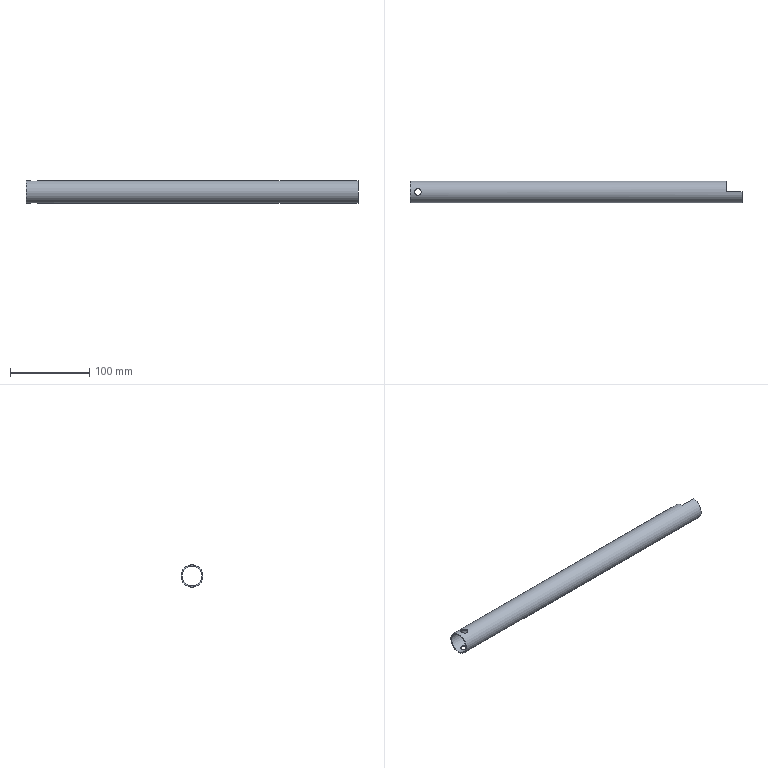Part | STEP file | GAS SHOCK A01W | 1 solid | 9 faces | box 420 x 28 x 28 mm | volume 51028 mm3 | plane 5 | cylinder 4 | commonest cylinder face diameters 8.5 x2 25 x1 28 x1